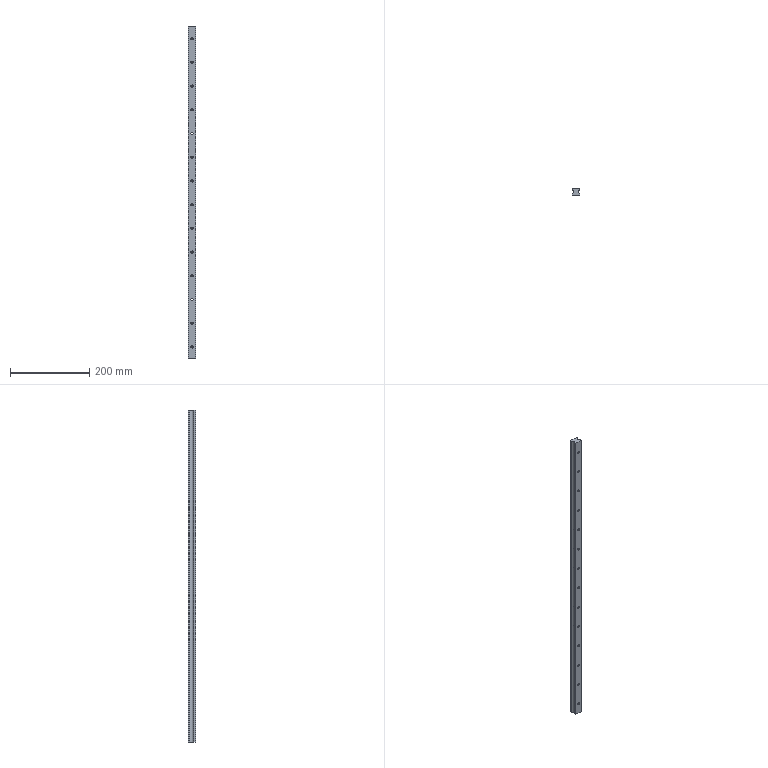Part | STEP file | Linear guide rail HG20 V1.201001 | 1 solid | 109 faces | box 20 x 18 x 840 mm | volume 247602 mm3 | cylinder 59 | cone 28 | plane 22 | commonest cylinder face diameters 5.5 x28 10 x28 10.692 x3